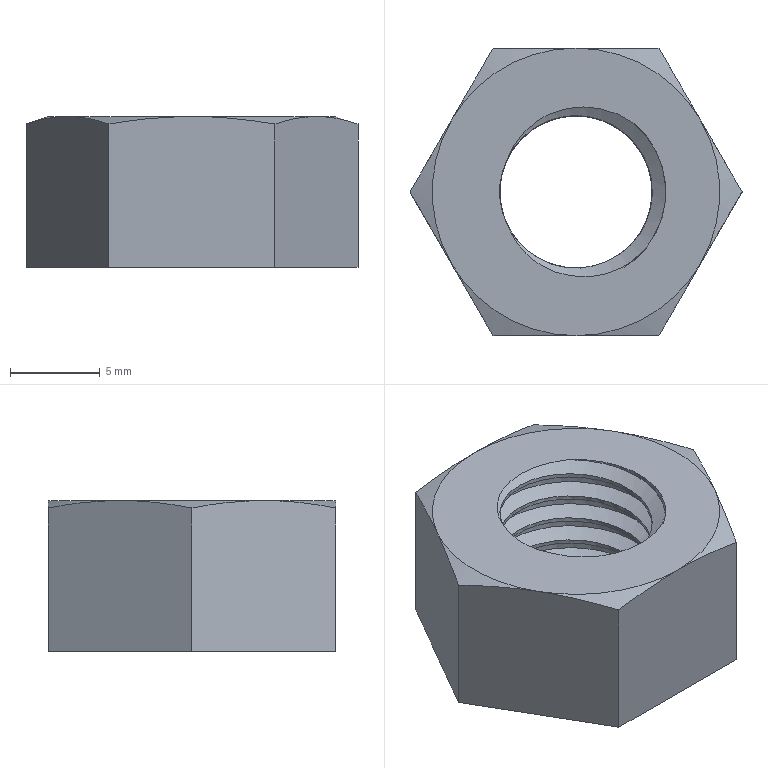Part | NX | features CHAMFER 1, CYLINDER 1, DATUM_CSYS 1, EXTRUDE 1, HOLE PACKAGE 1, SIMPLE HOLE 1, THREADS 1 | 1 solid | 19 faces | box 18.475 x 16 x 8.4 mm | volume 1288 mm3 | plane 9 | cone 6 | cylinder 2 | spline 2 | commonest cylinder face diameters 8.5 x1 10 x1
STEP:
#1=CARTESIAN_POINT('',(-4.619,-8.,0.));
#2=VERTEX_POINT('',#1);
#3=CARTESIAN_POINT('',(4.619,-8.,0.));
#4=VERTEX_POINT('',#3);
#5=CARTESIAN_POINT('',(-4.619,-8.,0.));
#6=DIRECTION('',(1.,0.,0.));
#7=VECTOR('',#6,1000.);
#8=LINE('',#5,#7);
#9=EDGE_CURVE('',#2,#4,#8,.T.);
#10=ORIENTED_EDGE('',*,*,#9,.F.);
#11=CARTESIAN_POINT('',(-9.238,0.,0.));
#12=VERTEX_POINT('',#11);
#13=CARTESIAN_POINT('',(-9.238,0.,0.));
#14=DIRECTION('',(0.5,-0.866,0.));
#15=VECTOR('',#14,1000.);
#16=LINE('',#13,#15);
#17=EDGE_CURVE('',#12,#2,#16,.T.);
#18=ORIENTED_EDGE('',*,*,#17,.F.);
#19=CARTESIAN_POINT('',(-4.619,8.,0.));
#20=VERTEX_POINT('',#19);
#21=CARTESIAN_POINT('',(-4.619,8.,0.));
#22=DIRECTION('',(-0.5,-0.866,0.));
#23=VECTOR('',#22,1000.);
#24=LINE('',#21,#23);
#25=EDGE_CURVE('',#20,#12,#24,.T.);
#26=ORIENTED_EDGE('',*,*,#25,.F.);
#27=CARTESIAN_POINT('',(4.619,8.,0.));
#28=VERTEX_POINT('',#27);
#29=CARTESIAN_POINT('',(4.619,8.,0.));
#30=DIRECTION('',(-1.,0.,0.));
#31=VECTOR('',#30,1000.);
#32=LINE('',#29,#31);
#33=EDGE_CURVE('',#28,#20,#32,.T.);
#34=ORIENTED_EDGE('',*,*,#33,.F.);
#35=CARTESIAN_POINT('',(9.238,0.,0.));
#36=VERTEX_POINT('',#35);
#37=CARTESIAN_POINT('',(9.238,0.,0.));
#38=DIRECTION('',(-0.5,0.866,0.));
#39=VECTOR('',#38,1000.);
#40=LINE('',#37,#39);
#41=EDGE_CURVE('',#36,#28,#40,.T.);
#42=ORIENTED_EDGE('',*,*,#41,.F.);
#43=CARTESIAN_POINT('',(4.619,-8.,0.));
#44=DIRECTION('',(0.5,0.866,0.));
#45=VECTOR('',#44,1000.);
#46=LINE('',#43,#45);
#47=EDGE_CURVE('',#4,#36,#46,.T.);
#48=ORIENTED_EDGE('',*,*,#47,.F.);
#49=EDGE_LOOP('',(#10,#18,#26,#34,#42,#48));
#50=FACE_BOUND('',#49,.T.);
#51=CARTESIAN_POINT('',(1.179,-4.083,0.));
#52=VERTEX_POINT('',#51);
#53=CARTESIAN_POINT('',(1.977,-3.762,0.));
#54=VERTEX_POINT('',#53);
#55=CARTESIAN_POINT('',(0.,0.,0.));
#56=DIRECTION('',(0.,0.,-1.));
#57=DIRECTION('',(-1.,0.,0.));
#58=AXIS2_PLACEMENT_3D('',#55,#56,#57);
#59=CIRCLE('',#58,4.25);
#60=EDGE_CURVE('',#52,#54,#59,.T.);
#61=ORIENTED_EDGE('',*,*,#60,.F.);
#62=CARTESIAN_POINT('',(1.202,-4.164,0.));
#63=VERTEX_POINT('',#62);
#64=CARTESIAN_POINT('',(0.,0.,0.));
#65=DIRECTION('',(0.2773,-0.9608,0.));
#66=VECTOR('',#65,1000.);
#67=LINE('',#64,#66);
#68=EDGE_CURVE('',#52,#63,#67,.T.);
#69=ORIENTED_EDGE('',*,*,#68,.T.);
#70=CARTESIAN_POINT('',(1.977,-3.762,0.));
#71=CARTESIAN_POINT('',(1.733,-3.923,0.));
#72=CARTESIAN_POINT('',(1.474,-4.056,0.));
#73=CARTESIAN_POINT('',(1.202,-4.164,0.));
#74=B_SPLINE_CURVE_WITH_KNOTS('',3,(#70,#71,#72,#73),.UNSPECIFIED.,.F.,.F.,(4,4),(0.0001042,0.0009768),.UNSPECIFIED.);
#75=EDGE_CURVE('',#54,#63,#74,.T.);
#76=ORIENTED_EDGE('',*,*,#75,.F.);
#77=EDGE_LOOP('',(#61,#69,#76));
#78=FACE_BOUND('',#77,.T.);
#79=CARTESIAN_POINT('',(0.,0.,0.));
#80=DIRECTION('',(0.,0.,-1.));
#81=DIRECTION('',(-1.,0.,0.));
#82=AXIS2_PLACEMENT_3D('',#79,#80,#81);
#83=PLANE('',#82);
#84=ADVANCED_FACE('',(#50,#78),#83,.T.);
#85=CARTESIAN_POINT('',(6.928,-4.,8.4));
#86=VERTEX_POINT('',#85);
#87=CARTESIAN_POINT('',(6.928,4.,8.4));
#88=VERTEX_POINT('',#87);
#89=CARTESIAN_POINT('',(0.,0.,8.4));
#90=DIRECTION('',(0.,0.,1.));
#91=DIRECTION('',(1.,0.,0.));
#92=AXIS2_PLACEMENT_3D('',#89,#90,#91);
#93=CIRCLE('',#92,8.);
#94=EDGE_CURVE('',#86,#88,#93,.T.);
#95=ORIENTED_EDGE('',*,*,#94,.F.);
#96=CARTESIAN_POINT('',(9.238,0.,7.987));
#97=VERTEX_POINT('',#96);
#98=CARTESIAN_POINT('',(6.928,-4.,8.4));
#99=CARTESIAN_POINT('',(7.698,-2.667,8.4));
#100=CARTESIAN_POINT('',(8.468,-1.333,8.244));
#101=CARTESIAN_POINT('',(9.238,0.,7.987));
#102=B_SPLINE_CURVE_WITH_KNOTS('',3,(#98,#99,#100,#101),.UNSPECIFIED.,.F.,.F.,(4,4),(0.004619,0.009238),.UNSPECIFIED.);
#103=EDGE_CURVE('',#86,#97,#102,.T.);
#104=ORIENTED_EDGE('',*,*,#103,.T.);
#105=CARTESIAN_POINT('',(9.238,0.,7.987));
#106=CARTESIAN_POINT('',(8.468,1.333,8.244));
#107=CARTESIAN_POINT('',(7.698,2.667,8.4));
#108=CARTESIAN_POINT('',(6.928,4.,8.4));
#109=B_SPLINE_CURVE_WITH_KNOTS('',3,(#105,#106,#107,#108),.UNSPECIFIED.,.F.,.F.,(4,4),(0.000000231,0.004619),.UNSPECIFIED.);
#110=EDGE_CURVE('',#97,#88,#109,.T.);
#111=ORIENTED_EDGE('',*,*,#110,.T.);
#112=EDGE_LOOP('',(#95,#104,#111));
#113=FACE_BOUND('',#112,.T.);
#114=CARTESIAN_POINT('',(0.,0.,7.4));
#115=DIRECTION('',(0.,0.,-1.));
#116=DIRECTION('',(-1.,0.,0.));
#117=AXIS2_PLACEMENT_3D('',#114,#115,#116);
#118=CONICAL_SURFACE('',#117,11.,1.249);
#119=ADVANCED_FACE('',(#113),#118,.T.);
#120=CARTESIAN_POINT('',(0.,-8.,8.4));
#121=VERTEX_POINT('',#120);
#122=CARTESIAN_POINT('',(0.,0.,8.4));
#123=DIRECTION('',(0.,0.,1.));
#124=DIRECTION('',(1.,0.,0.));
#125=AXIS2_PLACEMENT_3D('',#122,#123,#124);
#126=CIRCLE('',#125,8.);
#127=EDGE_CURVE('',#121,#86,#126,.T.);
#128=ORIENTED_EDGE('',*,*,#127,.F.);
#129=CARTESIAN_POINT('',(4.619,-8.,7.987));
#130=VERTEX_POINT('',#129);
#131=CARTESIAN_POINT('',(0.,-8.,8.4));
#132=CARTESIAN_POINT('',(1.544,-8.,8.4));
#133=CARTESIAN_POINT('',(3.083,-8.,8.243));
#134=CARTESIAN_POINT('',(4.619,-8.,7.987));
#135=B_SPLINE_CURVE_WITH_KNOTS('',3,(#131,#132,#133,#134),.UNSPECIFIED.,.F.,.F.,(4,4),(0.01252,0.01719),.UNSPECIFIED.);
#136=EDGE_CURVE('',#121,#130,#135,.T.);
#137=ORIENTED_EDGE('',*,*,#136,.T.);
#138=CARTESIAN_POINT('',(4.619,-8.,7.987));
#139=CARTESIAN_POINT('',(5.389,-6.667,8.244));
#140=CARTESIAN_POINT('',(6.158,-5.333,8.4));
#141=CARTESIAN_POINT('',(6.928,-4.,8.4));
#142=B_SPLINE_CURVE_WITH_KNOTS('',3,(#138,#139,#140,#141),.UNSPECIFIED.,.F.,.F.,(4,4),(0.000000231,0.004619),.UNSPECIFIED.);
#143=EDGE_CURVE('',#130,#86,#142,.T.);
#144=ORIENTED_EDGE('',*,*,#143,.T.);
#145=EDGE_LOOP('',(#128,#137,#144));
#146=FACE_BOUND('',#145,.T.);
#147=CARTESIAN_POINT('',(0.,0.,7.4));
#148=DIRECTION('',(0.,0.,-1.));
#149=DIRECTION('',(-1.,0.,0.));
#150=AXIS2_PLACEMENT_3D('',#147,#148,#149);
#151=CONICAL_SURFACE('',#150,11.,1.249);
#152=ADVANCED_FACE('',(#146),#151,.T.);
#153=CARTESIAN_POINT('',(-6.928,4.,8.4));
#154=VERTEX_POINT('',#153);
#155=CARTESIAN_POINT('',(-6.928,-4.,8.4));
#156=VERTEX_POINT('',#155);
#157=CARTESIAN_POINT('',(0.,0.,8.4));
#158=DIRECTION('',(0.,0.,1.));
#159=DIRECTION('',(1.,0.,0.));
#160=AXIS2_PLACEMENT_3D('',#157,#158,#159);
#161=CIRCLE('',#160,8.);
#162=EDGE_CURVE('',#154,#156,#161,.T.);
#163=ORIENTED_EDGE('',*,*,#162,.F.);
#164=CARTESIAN_POINT('',(-9.238,0.,7.987));
#165=VERTEX_POINT('',#164);
#166=CARTESIAN_POINT('',(-6.928,4.,8.4));
#167=CARTESIAN_POINT('',(-7.698,2.667,8.4));
#168=CARTESIAN_POINT('',(-8.468,1.333,8.244));
#169=CARTESIAN_POINT('',(-9.238,0.,7.987));
#170=B_SPLINE_CURVE_WITH_KNOTS('',3,(#166,#167,#168,#169),.UNSPECIFIED.,.F.,.F.,(4,4),(0.004619,0.009238),.UNSPECIFIED.);
#171=EDGE_CURVE('',#154,#165,#170,.T.);
#172=ORIENTED_EDGE('',*,*,#171,.T.);
#173=CARTESIAN_POINT('',(-9.238,0.,7.987));
#174=CARTESIAN_POINT('',(-8.468,-1.333,8.244));
#175=CARTESIAN_POINT('',(-7.698,-2.667,8.4));
#176=CARTESIAN_POINT('',(-6.928,-4.,8.4));
#177=B_SPLINE_CURVE_WITH_KNOTS('',3,(#173,#174,#175,#176),.UNSPECIFIED.,.F.,.F.,(4,4),(0.000000231,0.004619),.UNSPECIFIED.);
#178=EDGE_CURVE('',#165,#156,#177,.T.);
#179=ORIENTED_EDGE('',*,*,#178,.T.);
#180=EDGE_LOOP('',(#163,#172,#179));
#181=FACE_BOUND('',#180,.T.);
#182=CARTESIAN_POINT('',(0.,0.,7.4));
#183=DIRECTION('',(0.,0.,-1.));
#184=DIRECTION('',(-1.,0.,0.));
#185=AXIS2_PLACEMENT_3D('',#182,#183,#184);
#186=CONICAL_SURFACE('',#185,11.,1.249);
#187=ADVANCED_FACE('',(#181),#186,.T.);
#188=CARTESIAN_POINT('',(0.,8.,8.4));
#189=VERTEX_POINT('',#188);
#190=CARTESIAN_POINT('',(0.,0.,8.4));
#191=DIRECTION('',(0.,0.,1.));
#192=DIRECTION('',(1.,0.,0.));
#193=AXIS2_PLACEMENT_3D('',#190,#191,#192);
#194=CIRCLE('',#193,8.);
#195=EDGE_CURVE('',#189,#154,#194,.T.);
#196=ORIENTED_EDGE('',*,*,#195,.F.);
#197=CARTESIAN_POINT('',(-4.619,8.,7.987));
#198=VERTEX_POINT('',#197);
#199=CARTESIAN_POINT('',(-4.619,8.,7.987));
#200=CARTESIAN_POINT('',(-3.087,8.,8.243));
#201=CARTESIAN_POINT('',(-1.537,8.,8.4));
#202=CARTESIAN_POINT('',(0.,8.,8.4));
#203=B_SPLINE_CURVE_WITH_KNOTS('',3,(#199,#200,#201,#202),.UNSPECIFIED.,.F.,.F.,(4,4),(0.007866,0.01252),.UNSPECIFIED.);
#204=EDGE_CURVE('',#189,#198,#203,.F.);
#205=ORIENTED_EDGE('',*,*,#204,.T.);
#206=CARTESIAN_POINT('',(-4.619,8.,7.987));
#207=CARTESIAN_POINT('',(-5.389,6.667,8.244));
#208=CARTESIAN_POINT('',(-6.158,5.333,8.4));
#209=CARTESIAN_POINT('',(-6.928,4.,8.4));
#210=B_SPLINE_CURVE_WITH_KNOTS('',3,(#206,#207,#208,#209),.UNSPECIFIED.,.F.,.F.,(4,4),(0.000000231,0.004619),.UNSPECIFIED.);
#211=EDGE_CURVE('',#198,#154,#210,.T.);
#212=ORIENTED_EDGE('',*,*,#211,.T.);
#213=EDGE_LOOP('',(#196,#205,#212));
#214=FACE_BOUND('',#213,.T.);
#215=CARTESIAN_POINT('',(0.,0.,7.4));
#216=DIRECTION('',(0.,0.,-1.));
#217=DIRECTION('',(-1.,0.,0.));
#218=AXIS2_PLACEMENT_3D('',#215,#216,#217);
#219=CONICAL_SURFACE('',#218,11.,1.249);
#220=ADVANCED_FACE('',(#214),#219,.T.);
#221=CARTESIAN_POINT('',(0.,0.,8.4));
#222=DIRECTION('',(0.,0.,1.));
#223=DIRECTION('',(1.,0.,0.));
#224=AXIS2_PLACEMENT_3D('',#221,#222,#223);
#225=CIRCLE('',#224,8.);
#226=EDGE_CURVE('',#88,#189,#225,.T.);
#227=ORIENTED_EDGE('',*,*,#226,.F.);
#228=CARTESIAN_POINT('',(4.619,8.,7.987));
#229=VERTEX_POINT('',#228);
#230=CARTESIAN_POINT('',(6.928,4.,8.4));
#231=CARTESIAN_POINT('',(6.158,5.333,8.4));
#232=CARTESIAN_POINT('',(5.389,6.667,8.244));
#233=CARTESIAN_POINT('',(4.619,8.,7.987));
#234=B_SPLINE_CURVE_WITH_KNOTS('',3,(#230,#231,#232,#233),.UNSPECIFIED.,.F.,.F.,(4,4),(0.004619,0.009238),.UNSPECIFIED.);
#235=EDGE_CURVE('',#88,#229,#234,.T.);
#236=ORIENTED_EDGE('',*,*,#235,.T.);
#237=CARTESIAN_POINT('',(0.,8.,8.4));
#238=CARTESIAN_POINT('',(1.544,8.,8.4));
#239=CARTESIAN_POINT('',(3.083,8.,8.243));
#240=CARTESIAN_POINT('',(4.619,8.,7.987));
#241=B_SPLINE_CURVE_WITH_KNOTS('',3,(#237,#238,#239,#240),.UNSPECIFIED.,.F.,.F.,(4,4),(0.01252,0.01719),.UNSPECIFIED.);
#242=EDGE_CURVE('',#229,#189,#241,.F.);
#243=ORIENTED_EDGE('',*,*,#242,.T.);
#244=EDGE_LOOP('',(#227,#236,#243));
#245=FACE_BOUND('',#244,.T.);
#246=CARTESIAN_POINT('',(0.,0.,7.4));
#247=DIRECTION('',(0.,0.,-1.));
#248=DIRECTION('',(-1.,0.,0.));
#249=AXIS2_PLACEMENT_3D('',#246,#247,#248);
#250=CONICAL_SURFACE('',#249,11.,1.249);
#251=ADVANCED_FACE('',(#245),#250,.T.);
#252=CARTESIAN_POINT('',(3.228,3.819,8.4));
#253=VERTEX_POINT('',#252);
#254=CARTESIAN_POINT('',(-3.811,1.881,8.4));
#255=VERTEX_POINT('',#254);
#256=CARTESIAN_POINT('',(3.228,3.819,8.4));
#257=CARTESIAN_POINT('',(2.076,4.639,8.4));
#258=CARTESIAN_POINT('',(-0.936,5.227,8.4));
#259=CARTESIAN_POINT('',(-3.309,3.206,8.4));
#260=CARTESIAN_POINT('',(-3.811,1.881,8.4));
#261=B_SPLINE_CURVE_WITH_KNOTS('',3,(#256,#257,#258,#259,#260),.UNSPECIFIED.,.F.,.F.,(4,1,4),(0.00005872,0.004248,0.008437),.UNSPECIFIED.);
#262=EDGE_CURVE('',#253,#255,#261,.T.);
#263=ORIENTED_EDGE('',*,*,#262,.F.);
#264=CARTESIAN_POINT('',(3.228,-3.819,8.4));
#265=VERTEX_POINT('',#264);
#266=CARTESIAN_POINT('',(0.,0.,8.4));
#267=DIRECTION('',(0.,0.,1.));
#268=DIRECTION('',(1.,0.,0.));
#269=AXIS2_PLACEMENT_3D('',#266,#267,#268);
#270=CIRCLE('',#269,5.);
#271=EDGE_CURVE('',#265,#253,#270,.T.);
#272=ORIENTED_EDGE('',*,*,#271,.F.);
#273=CARTESIAN_POINT('',(-3.811,-1.881,8.4));
#274=VERTEX_POINT('',#273);
#275=CARTESIAN_POINT('',(-3.811,-1.881,8.4));
#276=CARTESIAN_POINT('',(-3.311,-3.202,8.4));
#277=CARTESIAN_POINT('',(-0.9386,-5.229,8.4));
#278=CARTESIAN_POINT('',(2.077,-4.638,8.4));
#279=CARTESIAN_POINT('',(3.228,-3.819,8.4));
#280=B_SPLINE_CURVE_WITH_KNOTS('',3,(#275,#276,#277,#278,#279),.UNSPECIFIED.,.F.,.F.,(4,1,4),(0.0001033,0.004312,0.00852),.UNSPECIFIED.);
#281=EDGE_CURVE('',#274,#265,#280,.T.);
#282=ORIENTED_EDGE('',*,*,#281,.F.);
#283=CARTESIAN_POINT('',(0.,0.,8.4));
#284=DIRECTION('',(0.,0.,-1.));
#285=DIRECTION('',(-1.,0.,0.));
#286=AXIS2_PLACEMENT_3D('',#283,#284,#285);
#287=CIRCLE('',#286,4.25);
#288=EDGE_CURVE('',#274,#255,#287,.T.);
#289=ORIENTED_EDGE('',*,*,#288,.T.);
#290=EDGE_LOOP('',(#263,#272,#282,#289));
#291=FACE_BOUND('',#290,.T.);
#292=ORIENTED_EDGE('',*,*,#226,.T.);
#293=ORIENTED_EDGE('',*,*,#195,.T.);
#294=ORIENTED_EDGE('',*,*,#162,.T.);
#295=CARTESIAN_POINT('',(0.,0.,8.4));
#296=DIRECTION('',(0.,0.,1.));
#297=DIRECTION('',(1.,0.,0.));
#298=AXIS2_PLACEMENT_3D('',#295,#296,#297);
#299=CIRCLE('',#298,8.);
#300=EDGE_CURVE('',#156,#121,#299,.T.);
#301=ORIENTED_EDGE('',*,*,#300,.T.);
#302=ORIENTED_EDGE('',*,*,#127,.T.);
#303=ORIENTED_EDGE('',*,*,#94,.T.);
#304=EDGE_LOOP('',(#292,#293,#294,#301,#302,#303));
#305=FACE_BOUND('',#304,.T.);
#306=CARTESIAN_POINT('',(0.,0.,8.4));
#307=DIRECTION('',(0.,0.,1.));
#308=DIRECTION('',(1.,0.,0.));
#309=AXIS2_PLACEMENT_3D('',#306,#307,#308);
#310=PLANE('',#309);
#311=ADVANCED_FACE('',(#291,#305),#310,.T.);
#312=CARTESIAN_POINT('',(-4.619,-8.,7.987));
#313=VERTEX_POINT('',#312);
#314=CARTESIAN_POINT('',(-6.928,-4.,8.4));
#315=CARTESIAN_POINT('',(-6.158,-5.333,8.4));
#316=CARTESIAN_POINT('',(-5.389,-6.667,8.244));
#317=CARTESIAN_POINT('',(-4.619,-8.,7.987));
#318=B_SPLINE_CURVE_WITH_KNOTS('',3,(#314,#315,#316,#317),.UNSPECIFIED.,.F.,.F.,(4,4),(0.004619,0.009238),.UNSPECIFIED.);
#319=EDGE_CURVE('',#156,#313,#318,.T.);
#320=ORIENTED_EDGE('',*,*,#319,.T.);
#321=CARTESIAN_POINT('',(-4.619,-8.,7.987));
#322=CARTESIAN_POINT('',(-3.087,-8.,8.243));
#323=CARTESIAN_POINT('',(-1.537,-8.,8.4));
#324=CARTESIAN_POINT('',(0.,-8.,8.4));
#325=B_SPLINE_CURVE_WITH_KNOTS('',3,(#321,#322,#323,#324),.UNSPECIFIED.,.F.,.F.,(4,4),(0.007866,0.01252),.UNSPECIFIED.);
#326=EDGE_CURVE('',#313,#121,#325,.T.);
#327=ORIENTED_EDGE('',*,*,#326,.T.);
#328=ORIENTED_EDGE('',*,*,#300,.F.);
#329=EDGE_LOOP('',(#320,#327,#328));
#330=FACE_BOUND('',#329,.T.);
#331=CARTESIAN_POINT('',(0.,0.,7.4));
#332=DIRECTION('',(0.,0.,-1.));
#333=DIRECTION('',(-1.,0.,0.));
#334=AXIS2_PLACEMENT_3D('',#331,#332,#333);
#335=CONICAL_SURFACE('',#334,11.,1.249);
#336=ADVANCED_FACE('',(#330),#335,.T.);
#337=ORIENTED_EDGE('',*,*,#326,.F.);
#338=CARTESIAN_POINT('',(-4.619,-8.,0.));
#339=DIRECTION('',(0.,0.,1.));
#340=VECTOR('',#339,1000.);
#341=LINE('',#338,#340);
#342=EDGE_CURVE('',#2,#313,#341,.T.);
#343=ORIENTED_EDGE('',*,*,#342,.F.);
#344=ORIENTED_EDGE('',*,*,#9,.T.);
#345=CARTESIAN_POINT('',(4.619,-8.,0.));
#346=DIRECTION('',(0.,0.,1.));
#347=VECTOR('',#346,1000.);
#348=LINE('',#345,#347);
#349=EDGE_CURVE('',#4,#130,#348,.T.);
#350=ORIENTED_EDGE('',*,*,#349,.T.);
#351=ORIENTED_EDGE('',*,*,#136,.F.);
#352=EDGE_LOOP('',(#337,#343,#344,#350,#351));
#353=FACE_BOUND('',#352,.T.);
#354=CARTESIAN_POINT('',(-4.619,-8.,0.));
#355=DIRECTION('',(0.,-1.,0.));
#356=DIRECTION('',(1.,0.,0.));
#357=AXIS2_PLACEMENT_3D('',#354,#355,#356);
#358=PLANE('',#357);
#359=ADVANCED_FACE('',(#353),#358,.T.);
#360=ORIENTED_EDGE('',*,*,#143,.F.);
#361=ORIENTED_EDGE('',*,*,#349,.F.);
#362=ORIENTED_EDGE('',*,*,#47,.T.);
#363=CARTESIAN_POINT('',(9.238,0.,0.));
#364=DIRECTION('',(0.,0.,1.));
#365=VECTOR('',#364,1000.);
#366=LINE('',#363,#365);
#367=EDGE_CURVE('',#36,#97,#366,.T.);
#368=ORIENTED_EDGE('',*,*,#367,.T.);
#369=ORIENTED_EDGE('',*,*,#103,.F.);
#370=EDGE_LOOP('',(#360,#361,#362,#368,#369));
#371=FACE_BOUND('',#370,.T.);
#372=CARTESIAN_POINT('',(4.619,-8.,0.));
#373=DIRECTION('',(0.866,-0.5,0.));
#374=DIRECTION('',(0.5,0.866,0.));
#375=AXIS2_PLACEMENT_3D('',#372,#373,#374);
#376=PLANE('',#375);
#377=ADVANCED_FACE('',(#371),#376,.T.);
#378=ORIENTED_EDGE('',*,*,#110,.F.);
#379=ORIENTED_EDGE('',*,*,#367,.F.);
#380=ORIENTED_EDGE('',*,*,#41,.T.);
#381=CARTESIAN_POINT('',(4.619,8.,0.));
#382=DIRECTION('',(0.,0.,1.));
#383=VECTOR('',#382,1000.);
#384=LINE('',#381,#383);
#385=EDGE_CURVE('',#28,#229,#384,.T.);
#386=ORIENTED_EDGE('',*,*,#385,.T.);
#387=ORIENTED_EDGE('',*,*,#235,.F.);
#388=EDGE_LOOP('',(#378,#379,#380,#386,#387));
#389=FACE_BOUND('',#388,.T.);
#390=CARTESIAN_POINT('',(9.238,0.,0.));
#391=DIRECTION('',(0.866,0.5,0.));
#392=DIRECTION('',(-0.5,0.866,0.));
#393=AXIS2_PLACEMENT_3D('',#390,#391,#392);
#394=PLANE('',#393);
#395=ADVANCED_FACE('',(#389),#394,.T.);
#396=ORIENTED_EDGE('',*,*,#242,.F.);
#397=ORIENTED_EDGE('',*,*,#385,.F.);
#398=ORIENTED_EDGE('',*,*,#33,.T.);
#399=CARTESIAN_POINT('',(-4.619,8.,0.));
#400=DIRECTION('',(0.,0.,1.));
#401=VECTOR('',#400,1000.);
#402=LINE('',#399,#401);
#403=EDGE_CURVE('',#20,#198,#402,.T.);
#404=ORIENTED_EDGE('',*,*,#403,.T.);
#405=ORIENTED_EDGE('',*,*,#204,.F.);
#406=EDGE_LOOP('',(#396,#397,#398,#404,#405));
#407=FACE_BOUND('',#406,.T.);
#408=CARTESIAN_POINT('',(4.619,8.,0.));
#409=DIRECTION('',(0.,1.,0.));
#410=DIRECTION('',(-1.,0.,0.));
#411=AXIS2_PLACEMENT_3D('',#408,#409,#410);
#412=PLANE('',#411);
#413=ADVANCED_FACE('',(#407),#412,.T.);
#414=ORIENTED_EDGE('',*,*,#211,.F.);
#415=ORIENTED_EDGE('',*,*,#403,.F.);
#416=ORIENTED_EDGE('',*,*,#25,.T.);
#417=CARTESIAN_POINT('',(-9.238,0.,0.));
#418=DIRECTION('',(0.,0.,1.));
#419=VECTOR('',#418,1000.);
#420=LINE('',#417,#419);
#421=EDGE_CURVE('',#12,#165,#420,.T.);
#422=ORIENTED_EDGE('',*,*,#421,.T.);
#423=ORIENTED_EDGE('',*,*,#171,.F.);
#424=EDGE_LOOP('',(#414,#415,#416,#422,#423));
#425=FACE_BOUND('',#424,.T.);
#426=CARTESIAN_POINT('',(-4.619,8.,0.));
#427=DIRECTION('',(-0.866,0.5,0.));
#428=DIRECTION('',(-0.5,-0.866,0.));
#429=AXIS2_PLACEMENT_3D('',#426,#427,#428);
#430=PLANE('',#429);
#431=ADVANCED_FACE('',(#425),#430,.T.);
#432=ORIENTED_EDGE('',*,*,#178,.F.);
#433=ORIENTED_EDGE('',*,*,#421,.F.);
#434=ORIENTED_EDGE('',*,*,#17,.T.);
#435=ORIENTED_EDGE('',*,*,#342,.T.);
#436=ORIENTED_EDGE('',*,*,#319,.F.);
#437=EDGE_LOOP('',(#432,#433,#434,#435,#436));
#438=FACE_BOUND('',#437,.T.);
#439=CARTESIAN_POINT('',(-9.238,0.,0.));
#440=DIRECTION('',(-0.866,-0.5,0.));
#441=DIRECTION('',(0.5,-0.866,0.));
#442=AXIS2_PLACEMENT_3D('',#439,#440,#441);
#443=PLANE('',#442);
#444=ADVANCED_FACE('',(#438),#443,.T.);
#445=ORIENTED_EDGE('',*,*,#60,.T.);
#446=CARTESIAN_POINT('',(1.977,-3.762,0.));
#447=CARTESIAN_POINT('',(3.369,-3.031,0.08878));
#448=CARTESIAN_POINT('',(5.184,0.06523,0.2621));
#449=CARTESIAN_POINT('',(2.302,4.66,0.5252));
#450=CARTESIAN_POINT('',(-3.109,4.164,0.7876));
#451=CARTESIAN_POINT('',(-5.12,-0.8825,1.05));
#452=CARTESIAN_POINT('',(-1.54,-4.961,1.313));
#453=CARTESIAN_POINT('',(3.72,-3.627,1.575));
#454=CARTESIAN_POINT('',(4.921,1.669,1.838));
#455=CARTESIAN_POINT('',(0.7438,5.142,2.1));
#456=CARTESIAN_POINT('',(-4.242,2.998,2.363));
#457=CARTESIAN_POINT('',(-4.599,-2.416,2.625));
#458=CARTESIAN_POINT('',(0.06565,-5.196,2.887));
#459=CARTESIAN_POINT('',(4.66,-2.297,3.15));
#460=CARTESIAN_POINT('',(4.163,3.107,3.413));
#461=CARTESIAN_POINT('',(-0.8754,5.121,3.675));
#462=CARTESIAN_POINT('',(-4.962,1.544,3.938));
#463=CARTESIAN_POINT('',(-3.626,-3.722,4.2));
#464=CARTESIAN_POINT('',(1.667,-4.92,4.462));
#465=CARTESIAN_POINT('',(5.141,-0.751,4.725));
#466=CARTESIAN_POINT('',(3.002,4.242,4.988));
#467=CARTESIAN_POINT('',(-2.418,4.599,5.25));
#468=CARTESIAN_POINT('',(-5.194,-0.06405,5.512));
#469=CARTESIAN_POINT('',(-2.304,-4.657,5.775));
#470=CARTESIAN_POINT('',(3.106,-4.166,6.038));
#471=CARTESIAN_POINT('',(5.121,0.8775,6.3));
#472=CARTESIAN_POINT('',(1.545,4.959,6.562));
#473=CARTESIAN_POINT('',(-3.716,3.631,6.825));
#474=CARTESIAN_POINT('',(-4.924,-1.666,7.087));
#475=CARTESIAN_POINT('',(-0.7415,-5.14,7.35));
#476=CARTESIAN_POINT('',(3.385,-3.361,7.569));
#477=CARTESIAN_POINT('',(4.458,-0.2923,7.744));
#478=CARTESIAN_POINT('',(3.959,2.073,7.875));
#479=CARTESIAN_POINT('',(2.29,3.838,8.006));
#480=CARTESIAN_POINT('',(-0.8428,4.688,8.181));
#481=CARTESIAN_POINT('',(-3.115,3.291,8.312));
#482=CARTESIAN_POINT('',(-3.811,1.881,8.4));
#483=B_SPLINE_CURVE_WITH_KNOTS('',3,(#446,#447,#448,#449,#450,#451,#452,#453,#454,#455,#456,#457,#458,#459,#460,#461,#462,#463,#464,#465,#466,#467,#468,#469,#470,#471,#472,#473,#474,#475,#476,#477,#478,#479,#480,#481,#482),.UNSPECIFIED.,.F.,.F.,(4,1,1,1,1,1,1,1,1,1,1,1,1,1,1,1,1,1,1,1,1,1,1,1,1,1,1,1,1,1,1,1,1,1,4),(0.,0.004678,0.009357,0.01404,0.01871,0.02339,0.02807,0.03275,0.03743,0.04211,0.04678,0.05146,0.05614,0.06082,0.0655,0.07018,0.07485,0.07953,0.08421,0.08889,0.09357,0.09825,0.1029,0.1076,0.1123,0.117,0.1216,0.1263,0.131,0.1357,0.138,0.1404,0.1427,0.145,0.1497),.UNSPECIFIED.);
#484=EDGE_CURVE('',#54,#255,#483,.T.);
#485=ORIENTED_EDGE('',*,*,#484,.T.);
#486=ORIENTED_EDGE('',*,*,#288,.F.);
#487=CARTESIAN_POINT('',(1.179,-4.083,1.233));
#488=VERTEX_POINT('',#487);
#489=CARTESIAN_POINT('',(-3.811,-1.881,8.4));
#490=CARTESIAN_POINT('',(-4.405,-0.6782,8.325));
#491=CARTESIAN_POINT('',(-4.36,2.267,8.176));
#492=CARTESIAN_POINT('',(-0.7489,4.865,7.952));
#493=CARTESIAN_POINT('',(3.482,3.477,7.728));
#494=CARTESIAN_POINT('',(4.862,-0.7537,7.504));
#495=CARTESIAN_POINT('',(2.267,-4.366,7.28));
#496=CARTESIAN_POINT('',(-2.178,-4.412,7.056));
#497=CARTESIAN_POINT('',(-4.847,-0.8513,6.832));
#498=CARTESIAN_POINT('',(-3.551,3.407,6.608));
#499=CARTESIAN_POINT('',(0.6494,4.877,6.384));
#500=CARTESIAN_POINT('',(4.315,2.363,6.16));
#501=CARTESIAN_POINT('',(4.458,-2.083,5.936));
#502=CARTESIAN_POINT('',(0.9539,-4.828,5.712));
#503=CARTESIAN_POINT('',(-3.331,-3.622,5.488));
#504=CARTESIAN_POINT('',(-4.889,0.5432,5.264));
#505=CARTESIAN_POINT('',(-2.456,4.263,5.04));
#506=CARTESIAN_POINT('',(1.988,4.502,4.816));
#507=CARTESIAN_POINT('',(4.806,1.056,4.592));
#508=CARTESIAN_POINT('',(3.692,-3.252,4.368));
#509=CARTESIAN_POINT('',(-0.4359,-4.9,4.144));
#510=CARTESIAN_POINT('',(-4.211,-2.547,3.92));
#511=CARTESIAN_POINT('',(-4.543,1.892,3.696));
#512=CARTESIAN_POINT('',(-1.158,4.782,3.472));
#513=CARTESIAN_POINT('',(3.17,3.762,3.248));
#514=CARTESIAN_POINT('',(4.909,-0.33,3.025));
#515=CARTESIAN_POINT('',(2.636,-4.156,2.8));
#516=CARTESIAN_POINT('',(-1.795,-4.582,2.577));
#517=CARTESIAN_POINT('',(-4.756,-1.26,2.352));
#518=CARTESIAN_POINT('',(-3.83,3.087,2.129));
#519=CARTESIAN_POINT('',(0.2245,4.915,1.905));
#520=CARTESIAN_POINT('',(4.101,2.724,1.68));
#521=CARTESIAN_POINT('',(4.61,-1.7,1.456));
#522=CARTESIAN_POINT('',(2.468,-3.711,1.308));
#523=CARTESIAN_POINT('',(1.179,-4.083,1.233));
#524=B_SPLINE_CURVE_WITH_KNOTS('',3,(#489,#490,#491,#492,#493,#494,#495,#496,#497,#498,#499,#500,#501,#502,#503,#504,#505,#506,#507,#508,#509,#510,#511,#512,#513,#514,#515,#516,#517,#518,#519,#520,#521,#522,#523),.UNSPECIFIED.,.F.,.F.,(4,1,1,1,1,1,1,1,1,1,1,1,1,1,1,1,1,1,1,1,1,1,1,1,1,1,1,1,1,1,1,1,4),(0.,0.003992,0.007984,0.01198,0.01597,0.01996,0.02395,0.02794,0.03194,0.03593,0.03992,0.04391,0.0479,0.0519,0.05589,0.05988,0.06387,0.06786,0.07185,0.07585,0.07984,0.08383,0.08782,0.09181,0.09581,0.0998,0.1038,0.1078,0.1118,0.1158,0.1198,0.1238,0.1277),.UNSPECIFIED.);
#525=EDGE_CURVE('',#274,#488,#524,.T.);
#526=ORIENTED_EDGE('',*,*,#525,.T.);
#527=CARTESIAN_POINT('',(1.179,-4.083,8.4));
#528=DIRECTION('',(0.,0.,-1.));
#529=VECTOR('',#528,1000.);
#530=LINE('',#527,#529);
#531=EDGE_CURVE('',#52,#488,#530,.F.);
#532=ORIENTED_EDGE('',*,*,#531,.F.);
#533=EDGE_LOOP('',(#445,#485,#486,#526,#532));
#534=FACE_BOUND('',#533,.T.);
#535=CARTESIAN_POINT('',(0.,0.,8.4));
#536=DIRECTION('',(0.,0.,-1.));
#537=DIRECTION('',(-1.,0.,0.));
#538=AXIS2_PLACEMENT_3D('',#535,#536,#537);
#539=CYLINDRICAL_SURFACE('',#538,4.25);
#540=ADVANCED_FACE('',(#534),#539,.F.);
#541=ORIENTED_EDGE('',*,*,#281,.T.);
#542=CARTESIAN_POINT('',(1.387,-4.804,0.7995));
#543=VERTEX_POINT('',#542);
#544=CARTESIAN_POINT('',(1.387,-4.804,0.7995));
#545=CARTESIAN_POINT('',(2.995,-4.34,0.8799));
#546=CARTESIAN_POINT('',(5.628,-1.718,1.036));
#547=CARTESIAN_POINT('',(4.513,3.797,1.275));
#548=CARTESIAN_POINT('',(-0.7286,5.849,1.512));
#549=CARTESIAN_POINT('',(-5.302,2.576,1.75));
#550=CARTESIAN_POINT('',(-5.048,-3.045,1.987));
#551=CARTESIAN_POINT('',(-0.1952,-5.892,2.225));
#552=CARTESIAN_POINT('',(4.835,-3.372,2.462));
#553=CARTESIAN_POINT('',(5.461,2.219,2.7));
#554=CARTESIAN_POINT('',(1.112,5.789,2.937));
#555=CARTESIAN_POINT('',(-4.25,4.085,3.175));
#556=CARTESIAN_POINT('',(-5.741,-1.34,3.412));
#557=CARTESIAN_POINT('',(-2.002,-5.545,3.65));
#558=CARTESIAN_POINT('',(3.56,-4.698,3.887));
#559=CARTESIAN_POINT('',(5.879,0.4273,4.125));
#560=CARTESIAN_POINT('',(2.843,5.164,4.362));
#561=CARTESIAN_POINT('',(-2.782,5.197,4.6));
#562=CARTESIAN_POINT('',(-5.874,0.4975,4.837));
#563=CARTESIAN_POINT('',(-3.617,-4.655,5.075));
#564=CARTESIAN_POINT('',(1.933,-5.568,5.312));
#565=CARTESIAN_POINT('',(5.723,-1.412,5.55));
#566=CARTESIAN_POINT('',(4.301,4.031,5.787));
#567=CARTESIAN_POINT('',(-1.038,5.803,6.024));
#568=CARTESIAN_POINT('',(-5.432,2.289,6.263));
#569=CARTESIAN_POINT('',(-4.878,-3.309,6.499));
#570=CARTESIAN_POINT('',(0.119,-5.894,6.738));
#571=CARTESIAN_POINT('',(5.008,-3.11,6.975));
#572=CARTESIAN_POINT('',(5.335,2.507,7.213));
#573=CARTESIAN_POINT('',(0.8021,5.84,7.45));
#574=CARTESIAN_POINT('',(-4.461,3.853,7.688));
#575=CARTESIAN_POINT('',(-5.662,-1.645,7.925));
#576=CARTESIAN_POINT('',(-1.701,-5.641,8.163));
#577=CARTESIAN_POINT('',(1.963,-4.887,8.32));
#578=CARTESIAN_POINT('',(3.228,-3.819,8.4));
#579=B_SPLINE_CURVE_WITH_KNOTS('',3,(#544,#545,#546,#547,#548,#549,#550,#551,#552,#553,#554,#555,#556,#557,#558,#559,#560,#561,#562,#563,#564,#565,#566,#567,#568,#569,#570,#571,#572,#573,#574,#575,#576,#577,#578),.UNSPECIFIED.,.F.,.F.,(4,1,1,1,1,1,1,1,1,1,1,1,1,1,1,1,1,1,1,1,1,1,1,1,1,1,1,1,1,1,1,1,4),(0.,0.004957,0.009913,0.01487,0.01983,0.02478,0.02974,0.0347,0.03965,0.04461,0.04957,0.05452,0.05948,0.06443,0.06939,0.07435,0.0793,0.08426,0.08922,0.09417,0.09913,0.1041,0.109,0.114,0.119,0.1239,0.1289,0.1338,0.1388,0.1437,0.1487,0.1537,0.1586),.UNSPECIFIED.);
#580=EDGE_CURVE('',#265,#543,#579,.F.);
#581=ORIENTED_EDGE('',*,*,#580,.T.);
#582=CARTESIAN_POINT('',(1.455,-5.041,0.657));
#583=CARTESIAN_POINT('',(1.176,-4.074,1.238));
#584=B_SPLINE_CURVE_WITH_KNOTS('',1,(#582,#583),.UNSPECIFIED.,.F.,.F.,(2,2),(0.,1.),.PIECEWISE_BEZIER_KNOTS.);
#585=EDGE_CURVE('',#543,#488,#584,.T.);
#586=ORIENTED_EDGE('',*,*,#585,.T.);
#587=ORIENTED_EDGE('',*,*,#525,.F.);
#588=EDGE_LOOP('',(#541,#581,#586,#587));
#589=FACE_BOUND('',#588,.T.);
#590=CARTESIAN_POINT('',(3.898,-3.139,8.443));
#591=CARTESIAN_POINT('',(3.785,-3.279,8.434));
#592=CARTESIAN_POINT('',(3.228,-3.901,8.394));
#593=CARTESIAN_POINT('',(1.965,-4.744,8.323));
#594=CARTESIAN_POINT('',(0.,-5.135,8.23));
#595=CARTESIAN_POINT('',(-1.965,-4.744,8.136));
#596=CARTESIAN_POINT('',(-3.631,-3.631,8.042));
#597=CARTESIAN_POINT('',(-4.744,-1.965,7.948));
#598=CARTESIAN_POINT('',(-5.135,0.,7.855));
#599=CARTESIAN_POINT('',(-4.744,1.965,7.761));
#600=CARTESIAN_POINT('',(-3.631,3.631,7.667));
#601=CARTESIAN_POINT('',(-1.965,4.744,7.573));
#602=CARTESIAN_POINT('',(0.,5.135,7.48));
#603=CARTESIAN_POINT('',(1.965,4.744,7.386));
#604=CARTESIAN_POINT('',(3.631,3.631,7.292));
#605=CARTESIAN_POINT('',(4.744,1.965,7.198));
#606=CARTESIAN_POINT('',(5.135,0.,7.105));
#607=CARTESIAN_POINT('',(4.744,-1.965,7.011));
#608=CARTESIAN_POINT('',(3.631,-3.631,6.917));
#609=CARTESIAN_POINT('',(1.965,-4.744,6.823));
#610=CARTESIAN_POINT('',(0.,-5.135,6.73));
#611=CARTESIAN_POINT('',(-1.965,-4.744,6.636));
#612=CARTESIAN_POINT('',(-3.631,-3.631,6.542));
#613=CARTESIAN_POINT('',(-4.744,-1.965,6.448));
#614=CARTESIAN_POINT('',(-5.135,0.,6.355));
#615=CARTESIAN_POINT('',(-4.744,1.965,6.261));
#616=CARTESIAN_POINT('',(-3.631,3.631,6.167));
#617=CARTESIAN_POINT('',(-1.965,4.744,6.073));
#618=CARTESIAN_POINT('',(0.,5.135,5.98));
#619=CARTESIAN_POINT('',(1.965,4.744,5.886));
#620=CARTESIAN_POINT('',(3.631,3.631,5.792));
#621=CARTESIAN_POINT('',(4.744,1.965,5.698));
#622=CARTESIAN_POINT('',(5.135,0.,5.605));
#623=CARTESIAN_POINT('',(4.744,-1.965,5.511));
#624=CARTESIAN_POINT('',(3.631,-3.631,5.417));
#625=CARTESIAN_POINT('',(1.965,-4.744,5.323));
#626=CARTESIAN_POINT('',(0.,-5.135,5.23));
#627=CARTESIAN_POINT('',(-1.965,-4.744,5.136));
#628=CARTESIAN_POINT('',(-3.631,-3.631,5.042));
#629=CARTESIAN_POINT('',(-4.744,-1.965,4.948));
#630=CARTESIAN_POINT('',(-5.135,0.,4.855));
#631=CARTESIAN_POINT('',(-4.744,1.965,4.761));
#632=CARTESIAN_POINT('',(-3.631,3.631,4.667));
#633=CARTESIAN_POINT('',(-1.965,4.744,4.573));
#634=CARTESIAN_POINT('',(0.,5.135,4.48));
#635=CARTESIAN_POINT('',(1.965,4.744,4.386));
#636=CARTESIAN_POINT('',(3.631,3.631,4.292));
#637=CARTESIAN_POINT('',(4.744,1.965,4.198));
#638=CARTESIAN_POINT('',(5.135,0.,4.105));
#639=CARTESIAN_POINT('',(4.744,-1.965,4.011));
#640=CARTESIAN_POINT('',(3.631,-3.631,3.917));
#641=CARTESIAN_POINT('',(1.965,-4.744,3.823));
#642=CARTESIAN_POINT('',(0.,-5.135,3.73));
#643=CARTESIAN_POINT('',(-1.965,-4.744,3.636));
#644=CARTESIAN_POINT('',(-3.631,-3.631,3.542));
#645=CARTESIAN_POINT('',(-4.744,-1.965,3.448));
#646=CARTESIAN_POINT('',(-5.135,0.,3.355));
#647=CARTESIAN_POINT('',(-4.744,1.965,3.261));
#648=CARTESIAN_POINT('',(-3.631,3.631,3.167));
#649=CARTESIAN_POINT('',(-1.965,4.744,3.073));
#650=CARTESIAN_POINT('',(0.,5.135,2.98));
#651=CARTESIAN_POINT('',(1.965,4.744,2.886));
#652=CARTESIAN_POINT('',(3.631,3.631,2.792));
#653=CARTESIAN_POINT('',(4.744,1.965,2.698));
#654=CARTESIAN_POINT('',(5.135,0.,2.605));
#655=CARTESIAN_POINT('',(4.744,-1.965,2.511));
#656=CARTESIAN_POINT('',(3.631,-3.631,2.417));
#657=CARTESIAN_POINT('',(1.965,-4.744,2.323));
#658=CARTESIAN_POINT('',(0.,-5.135,2.23));
#659=CARTESIAN_POINT('',(-1.965,-4.744,2.136));
#660=CARTESIAN_POINT('',(-3.631,-3.631,2.042));
#661=CARTESIAN_POINT('',(-4.744,-1.965,1.948));
#662=CARTESIAN_POINT('',(-5.135,0.,1.855));
#663=CARTESIAN_POINT('',(-4.744,1.965,1.761));
#664=CARTESIAN_POINT('',(-3.631,3.631,1.667));
#665=CARTESIAN_POINT('',(-1.965,4.744,1.573));
#666=CARTESIAN_POINT('',(0.,5.135,1.48));
#667=CARTESIAN_POINT('',(1.965,4.744,1.386));
#668=CARTESIAN_POINT('',(3.631,3.631,1.292));
#669=CARTESIAN_POINT('',(4.744,1.965,1.198));
#670=CARTESIAN_POINT('',(5.135,0.,1.105));
#671=CARTESIAN_POINT('',(4.744,-1.965,1.011));
#672=CARTESIAN_POINT('',(3.631,-3.631,0.9172));
#673=CARTESIAN_POINT('',(2.363,-4.479,0.8458));
#674=CARTESIAN_POINT('',(1.567,-4.757,0.8057));
#675=CARTESIAN_POINT('',(1.388,-4.808,0.7968));
#676=CARTESIAN_POINT('',(3.306,-2.663,8.881));
#677=CARTESIAN_POINT('',(3.211,-2.781,8.873));
#678=CARTESIAN_POINT('',(2.738,-3.309,8.833));
#679=CARTESIAN_POINT('',(1.667,-4.024,8.762));
#680=CARTESIAN_POINT('',(0.,-4.356,8.668));
#681=CARTESIAN_POINT('',(-1.667,-4.024,8.575));
#682=CARTESIAN_POINT('',(-3.08,-3.08,8.481));
#683=CARTESIAN_POINT('',(-4.024,-1.667,8.387));
#684=CARTESIAN_POINT('',(-4.356,0.,8.293));
#685=CARTESIAN_POINT('',(-4.024,1.667,8.2));
#686=CARTESIAN_POINT('',(-3.08,3.08,8.106));
#687=CARTESIAN_POINT('',(-1.667,4.024,8.012));
#688=CARTESIAN_POINT('',(0.,4.356,7.918));
#689=CARTESIAN_POINT('',(1.667,4.024,7.825));
#690=CARTESIAN_POINT('',(3.08,3.08,7.731));
#691=CARTESIAN_POINT('',(4.024,1.667,7.637));
#692=CARTESIAN_POINT('',(4.356,0.,7.543));
#693=CARTESIAN_POINT('',(4.024,-1.667,7.45));
#694=CARTESIAN_POINT('',(3.08,-3.08,7.356));
#695=CARTESIAN_POINT('',(1.667,-4.024,7.262));
#696=CARTESIAN_POINT('',(0.,-4.356,7.168));
#697=CARTESIAN_POINT('',(-1.667,-4.024,7.075));
#698=CARTESIAN_POINT('',(-3.08,-3.08,6.981));
#699=CARTESIAN_POINT('',(-4.024,-1.667,6.887));
#700=CARTESIAN_POINT('',(-4.356,0.,6.793));
#701=CARTESIAN_POINT('',(-4.024,1.667,6.7));
#702=CARTESIAN_POINT('',(-3.08,3.08,6.606));
#703=CARTESIAN_POINT('',(-1.667,4.024,6.512));
#704=CARTESIAN_POINT('',(0.,4.356,6.418));
#705=CARTESIAN_POINT('',(1.667,4.024,6.325));
#706=CARTESIAN_POINT('',(3.08,3.08,6.231));
#707=CARTESIAN_POINT('',(4.024,1.667,6.137));
#708=CARTESIAN_POINT('',(4.356,0.,6.043));
#709=CARTESIAN_POINT('',(4.024,-1.667,5.95));
#710=CARTESIAN_POINT('',(3.08,-3.08,5.856));
#711=CARTESIAN_POINT('',(1.667,-4.024,5.762));
#712=CARTESIAN_POINT('',(0.,-4.356,5.668));
#713=CARTESIAN_POINT('',(-1.667,-4.024,5.575));
#714=CARTESIAN_POINT('',(-3.08,-3.08,5.481));
#715=CARTESIAN_POINT('',(-4.024,-1.667,5.387));
#716=CARTESIAN_POINT('',(-4.356,0.,5.293));
#717=CARTESIAN_POINT('',(-4.024,1.667,5.2));
#718=CARTESIAN_POINT('',(-3.08,3.08,5.106));
#719=CARTESIAN_POINT('',(-1.667,4.024,5.012));
#720=CARTESIAN_POINT('',(0.,4.356,4.918));
#721=CARTESIAN_POINT('',(1.667,4.024,4.825));
#722=CARTESIAN_POINT('',(3.08,3.08,4.731));
#723=CARTESIAN_POINT('',(4.024,1.667,4.637));
#724=CARTESIAN_POINT('',(4.356,0.,4.543));
#725=CARTESIAN_POINT('',(4.024,-1.667,4.45));
#726=CARTESIAN_POINT('',(3.08,-3.08,4.356));
#727=CARTESIAN_POINT('',(1.667,-4.024,4.262));
#728=CARTESIAN_POINT('',(0.,-4.356,4.168));
#729=CARTESIAN_POINT('',(-1.667,-4.024,4.075));
#730=CARTESIAN_POINT('',(-3.08,-3.08,3.981));
#731=CARTESIAN_POINT('',(-4.024,-1.667,3.887));
#732=CARTESIAN_POINT('',(-4.356,0.,3.793));
#733=CARTESIAN_POINT('',(-4.024,1.667,3.7));
#734=CARTESIAN_POINT('',(-3.08,3.08,3.606));
#735=CARTESIAN_POINT('',(-1.667,4.024,3.512));
#736=CARTESIAN_POINT('',(0.,4.356,3.418));
#737=CARTESIAN_POINT('',(1.667,4.024,3.325));
#738=CARTESIAN_POINT('',(3.08,3.08,3.231));
#739=CARTESIAN_POINT('',(4.024,1.667,3.137));
#740=CARTESIAN_POINT('',(4.356,0.,3.043));
#741=CARTESIAN_POINT('',(4.024,-1.667,2.95));
#742=CARTESIAN_POINT('',(3.08,-3.08,2.856));
#743=CARTESIAN_POINT('',(1.667,-4.024,2.762));
#744=CARTESIAN_POINT('',(0.,-4.356,2.668));
#745=CARTESIAN_POINT('',(-1.667,-4.024,2.575));
#746=CARTESIAN_POINT('',(-3.08,-3.08,2.481));
#747=CARTESIAN_POINT('',(-4.024,-1.667,2.387));
#748=CARTESIAN_POINT('',(-4.356,0.,2.293));
#749=CARTESIAN_POINT('',(-4.024,1.667,2.2));
#750=CARTESIAN_POINT('',(-3.08,3.08,2.106));
#751=CARTESIAN_POINT('',(-1.667,4.024,2.012));
#752=CARTESIAN_POINT('',(0.,4.356,1.918));
#753=CARTESIAN_POINT('',(1.667,4.024,1.825));
#754=CARTESIAN_POINT('',(3.08,3.08,1.731));
#755=CARTESIAN_POINT('',(4.024,1.667,1.637));
#756=CARTESIAN_POINT('',(4.356,0.,1.543));
#757=CARTESIAN_POINT('',(4.024,-1.667,1.45));
#758=CARTESIAN_POINT('',(3.08,-3.08,1.356));
#759=CARTESIAN_POINT('',(2.004,-3.799,1.284));
#760=CARTESIAN_POINT('',(1.329,-4.035,1.244));
#761=CARTESIAN_POINT('',(1.177,-4.079,1.235));
#762=B_SPLINE_SURFACE_WITH_KNOTS('',1,3,((#590,#591,#592,#593,#594,#595,#596,#597,#598,#599,#600,#601,#602,#603,#604,#605,#606,#607,#608,#609,#610,#611,#612,#613,#614,#615,#616,#617,#618,#619,#620,#621,#622,#623,#624,#625,#626,#627,#628,#629,#630,#631,#632,#633,#634,#635,#636,#637,#638,#639,#640,#641,#642,#643,#644,#645,#646,#647,#648,#649,#650,#651,#652,#653,#654,#655,#656,#657,#658,#659,#660,#661,#662,#663,#664,#665,#666,#667,#668,#669,#670,#671,#672,#673,#674,#675),(#676,#677,#678,#679,#680,#681,#682,#683,#684,#685,#686,#687,#688,#689,#690,#691,#692,#693,#694,#695,#696,#697,#698,#699,#700,#701,#702,#703,#704,#705,#706,#707,#708,#709,#710,#711,#712,#713,#714,#715,#716,#717,#718,#719,#720,#721,#722,#723,#724,#725,#726,#727,#728,#729,#730,#731,#732,#733,#734,#735,#736,#737,#738,#739,#740,#741,#742,#743,#744,#745,#746,#747,#748,#749,#750,#751,#752,#753,#754,#755,#756,#757,#758,#759,#760,#761)),.RULED_SURF.,.F.,.F.,.F.,(2,2),(4,1,1,1,1,1,1,1,1,1,1,1,1,1,1,1,1,1,1,1,1,1,1,1,1,1,1,1,1,1,1,1,1,1,1,1,1,1,1,1,1,1,1,1,1,1,1,1,1,1,1,1,1,1,1,1,1,1,1,1,1,1,1,1,1,1,1,1,1,1,1,1,1,1,1,1,1,1,1,1,1,1,1,4),(0.2404,0.9947),(0.1066,0.1095,0.1205,0.1315,0.1424,0.1534,0.1643,0.1753,0.1862,0.1972,0.2081,0.2191,0.2301,0.241,0.252,0.2629,0.2739,0.2848,0.2958,0.3067,0.3177,0.3286,0.3396,0.3506,0.3615,0.3725,0.3834,0.3944,0.4053,0.4163,0.4272,0.4382,0.4491,0.4601,0.4711,0.482,0.493,0.5039,0.5149,0.5258,0.5368,0.5477,0.5587,0.5696,0.5806,0.5916,0.6025,0.6135,0.6244,0.6354,0.6463,0.6573,0.6682,0.6792,0.6902,0.7011,0.7121,0.723,0.734,0.7449,0.7559,0.7668,0.7778,0.7887,0.7997,0.8107,0.8216,0.8326,0.8435,0.8545,0.8654,0.8764,0.8873,0.8983,0.9092,0.9202,0.9312,0.9421,0.9531,0.964,0.975,0.9859,0.9969,1.),.UNSPECIFIED.);
#763=ADVANCED_FACE('',(#589),#762,.F.);
#764=ORIENTED_EDGE('',*,*,#531,.T.);
#765=ORIENTED_EDGE('',*,*,#585,.F.);
#766=CARTESIAN_POINT('',(1.387,-4.804,0.3847));
#767=VERTEX_POINT('',#766);
#768=CARTESIAN_POINT('',(1.387,-4.804,9.15));
#769=DIRECTION('',(0.,0.,-1.));
#770=VECTOR('',#769,1000.);
#771=LINE('',#768,#770);
#772=EDGE_CURVE('',#767,#543,#771,.F.);
#773=ORIENTED_EDGE('',*,*,#772,.F.);
#774=CARTESIAN_POINT('',(1.176,-4.074,-0.05427));
#775=CARTESIAN_POINT('',(1.455,-5.041,0.5272));
#776=B_SPLINE_CURVE_WITH_KNOTS('',1,(#774,#775),.UNSPECIFIED.,.F.,.F.,(2,2),(0.,1.),.PIECEWISE_BEZIER_KNOTS.);
#777=EDGE_CURVE('',#63,#767,#776,.T.);
#778=ORIENTED_EDGE('',*,*,#777,.F.);
#779=ORIENTED_EDGE('',*,*,#68,.F.);
#780=EDGE_LOOP('',(#764,#765,#773,#778,#779));
#781=FACE_BOUND('',#780,.T.);
#782=CARTESIAN_POINT('',(1.176,-4.074,0.5921));
#783=DIRECTION('',(0.9608,0.2773,0.));
#784=DIRECTION('',(-0.2773,0.9608,0.));
#785=AXIS2_PLACEMENT_3D('',#782,#783,#784);
#786=PLANE('',#785);
#787=ADVANCED_FACE('',(#781),#786,.T.);
#788=ORIENTED_EDGE('',*,*,#262,.T.);
#789=ORIENTED_EDGE('',*,*,#484,.F.);
#790=ORIENTED_EDGE('',*,*,#75,.T.);
#791=ORIENTED_EDGE('',*,*,#777,.T.);
#792=CARTESIAN_POINT('',(3.228,3.819,8.4));
#793=CARTESIAN_POINT('',(4.561,2.692,8.316));
#794=CARTESIAN_POINT('',(5.903,-1.072,8.15));
#795=CARTESIAN_POINT('',(2.011,-5.659,7.899));
#796=CARTESIAN_POINT('',(-3.906,-4.561,7.648));
#797=CARTESIAN_POINT('',(-5.9,1.114,7.398));
#798=CARTESIAN_POINT('',(-1.973,5.67,7.147));
#799=CARTESIAN_POINT('',(3.932,4.537,6.897));
#800=CARTESIAN_POINT('',(5.893,-1.148,6.647));
#801=CARTESIAN_POINT('',(1.942,-5.681,6.396));
#802=CARTESIAN_POINT('',(-3.957,-4.515,6.146));
#803=CARTESIAN_POINT('',(-5.887,1.181,5.895));
#804=CARTESIAN_POINT('',(-1.909,5.693,5.645));
#805=CARTESIAN_POINT('',(3.986,4.491,5.394));
#806=CARTESIAN_POINT('',(5.879,-1.22,5.144));
#807=CARTESIAN_POINT('',(1.871,-5.705,4.893));
#808=CARTESIAN_POINT('',(-4.013,-4.465,4.643));
#809=CARTESIAN_POINT('',(-5.871,1.254,4.392));
#810=CARTESIAN_POINT('',(-1.839,5.715,4.142));
#811=CARTESIAN_POINT('',(4.038,4.443,3.891));
#812=CARTESIAN_POINT('',(5.865,-1.286,3.641));
#813=CARTESIAN_POINT('',(1.807,-5.726,3.39));
#814=CARTESIAN_POINT('',(-4.065,-4.419,3.14));
#815=CARTESIAN_POINT('',(-5.857,1.325,2.89));
#816=CARTESIAN_POINT('',(-1.769,5.738,2.639));
#817=CARTESIAN_POINT('',(4.093,4.393,2.388));
#818=CARTESIAN_POINT('',(5.848,-1.359,2.138));
#819=CARTESIAN_POINT('',(1.736,-5.747,1.888));
#820=CARTESIAN_POINT('',(-4.117,-4.37,1.637));
#821=CARTESIAN_POINT('',(-5.84,1.392,1.387));
#822=CARTESIAN_POINT('',(-1.705,5.757,1.136));
#823=CARTESIAN_POINT('',(4.147,4.347,0.8856));
#824=CARTESIAN_POINT('',(5.819,-1.433,0.6352));
#825=CARTESIAN_POINT('',(3.083,-4.314,0.4685));
#826=CARTESIAN_POINT('',(1.387,-4.804,0.3847));
#827=B_SPLINE_CURVE_WITH_KNOTS('',3,(#792,#793,#794,#795,#796,#797,#798,#799,#800,#801,#802,#803,#804,#805,#806,#807,#808,#809,#810,#811,#812,#813,#814,#815,#816,#817,#818,#819,#820,#821,#822,#823,#824,#825,#826),.UNSPECIFIED.,.F.,.F.,(4,1,1,1,1,1,1,1,1,1,1,1,1,1,1,1,1,1,1,1,1,1,1,1,1,1,1,1,1,1,1,1,4),(0.01132,0.01655,0.02178,0.027,0.03223,0.03746,0.04269,0.04791,0.05314,0.05837,0.06359,0.06882,0.07405,0.07927,0.0845,0.08973,0.09496,0.1002,0.1054,0.1106,0.1159,0.1211,0.1263,0.1315,0.1368,0.142,0.1472,0.1525,0.1577,0.1629,0.1681,0.1734,0.1786),.UNSPECIFIED.);
#828=EDGE_CURVE('',#767,#253,#827,.F.);
#829=ORIENTED_EDGE('',*,*,#828,.T.);
#830=EDGE_LOOP('',(#788,#789,#790,#791,#829));
#831=FACE_BOUND('',#830,.T.);
#832=CARTESIAN_POINT('',(-4.117,1.035,8.448));
#833=CARTESIAN_POINT('',(-4.067,1.236,8.436));
#834=CARTESIAN_POINT('',(-3.827,1.962,8.393));
#835=CARTESIAN_POINT('',(-3.08,3.08,8.319));
#836=CARTESIAN_POINT('',(-1.667,4.024,8.225));
#837=CARTESIAN_POINT('',(0.,4.356,8.132));
#838=CARTESIAN_POINT('',(1.667,4.024,8.038));
#839=CARTESIAN_POINT('',(3.08,3.08,7.944));
#840=CARTESIAN_POINT('',(4.024,1.667,7.85));
#841=CARTESIAN_POINT('',(4.356,0.,7.757));
#842=CARTESIAN_POINT('',(4.024,-1.667,7.663));
#843=CARTESIAN_POINT('',(3.08,-3.08,7.569));
#844=CARTESIAN_POINT('',(1.667,-4.024,7.475));
#845=CARTESIAN_POINT('',(0.,-4.356,7.382));
#846=CARTESIAN_POINT('',(-1.667,-4.024,7.288));
#847=CARTESIAN_POINT('',(-3.08,-3.08,7.194));
#848=CARTESIAN_POINT('',(-4.024,-1.667,7.1));
#849=CARTESIAN_POINT('',(-4.356,0.,7.007));
#850=CARTESIAN_POINT('',(-4.024,1.667,6.913));
#851=CARTESIAN_POINT('',(-3.08,3.08,6.819));
#852=CARTESIAN_POINT('',(-1.667,4.024,6.725));
#853=CARTESIAN_POINT('',(0.,4.356,6.632));
#854=CARTESIAN_POINT('',(1.667,4.024,6.538));
#855=CARTESIAN_POINT('',(3.08,3.08,6.444));
#856=CARTESIAN_POINT('',(4.024,1.667,6.35));
#857=CARTESIAN_POINT('',(4.356,0.,6.257));
#858=CARTESIAN_POINT('',(4.024,-1.667,6.163));
#859=CARTESIAN_POINT('',(3.08,-3.08,6.069));
#860=CARTESIAN_POINT('',(1.667,-4.024,5.975));
#861=CARTESIAN_POINT('',(0.,-4.356,5.882));
#862=CARTESIAN_POINT('',(-1.667,-4.024,5.788));
#863=CARTESIAN_POINT('',(-3.08,-3.08,5.694));
#864=CARTESIAN_POINT('',(-4.024,-1.667,5.6));
#865=CARTESIAN_POINT('',(-4.356,0.,5.507));
#866=CARTESIAN_POINT('',(-4.024,1.667,5.413));
#867=CARTESIAN_POINT('',(-3.08,3.08,5.319));
#868=CARTESIAN_POINT('',(-1.667,4.024,5.225));
#869=CARTESIAN_POINT('',(0.,4.356,5.132));
#870=CARTESIAN_POINT('',(1.667,4.024,5.038));
#871=CARTESIAN_POINT('',(3.08,3.08,4.944));
#872=CARTESIAN_POINT('',(4.024,1.667,4.85));
#873=CARTESIAN_POINT('',(4.356,0.,4.757));
#874=CARTESIAN_POINT('',(4.024,-1.667,4.663));
#875=CARTESIAN_POINT('',(3.08,-3.08,4.569));
#876=CARTESIAN_POINT('',(1.667,-4.024,4.475));
#877=CARTESIAN_POINT('',(0.,-4.356,4.382));
#878=CARTESIAN_POINT('',(-1.667,-4.024,4.288));
#879=CARTESIAN_POINT('',(-3.08,-3.08,4.194));
#880=CARTESIAN_POINT('',(-4.024,-1.667,4.1));
#881=CARTESIAN_POINT('',(-4.356,0.,4.007));
#882=CARTESIAN_POINT('',(-4.024,1.667,3.913));
#883=CARTESIAN_POINT('',(-3.08,3.08,3.819));
#884=CARTESIAN_POINT('',(-1.667,4.024,3.725));
#885=CARTESIAN_POINT('',(0.,4.356,3.632));
#886=CARTESIAN_POINT('',(1.667,4.024,3.538));
#887=CARTESIAN_POINT('',(3.08,3.08,3.444));
#888=CARTESIAN_POINT('',(4.024,1.667,3.35));
#889=CARTESIAN_POINT('',(4.356,0.,3.257));
#890=CARTESIAN_POINT('',(4.024,-1.667,3.163));
#891=CARTESIAN_POINT('',(3.08,-3.08,3.069));
#892=CARTESIAN_POINT('',(1.667,-4.024,2.975));
#893=CARTESIAN_POINT('',(0.,-4.356,2.882));
#894=CARTESIAN_POINT('',(-1.667,-4.024,2.788));
#895=CARTESIAN_POINT('',(-3.08,-3.08,2.694));
#896=CARTESIAN_POINT('',(-4.024,-1.667,2.6));
#897=CARTESIAN_POINT('',(-4.356,0.,2.507));
#898=CARTESIAN_POINT('',(-4.024,1.667,2.413));
#899=CARTESIAN_POINT('',(-3.08,3.08,2.319));
#900=CARTESIAN_POINT('',(-1.667,4.024,2.225));
#901=CARTESIAN_POINT('',(0.,4.356,2.132));
#902=CARTESIAN_POINT('',(1.667,4.024,2.038));
#903=CARTESIAN_POINT('',(3.08,3.08,1.944));
#904=CARTESIAN_POINT('',(4.024,1.667,1.85));
#905=CARTESIAN_POINT('',(4.356,0.,1.757));
#906=CARTESIAN_POINT('',(4.024,-1.667,1.663));
#907=CARTESIAN_POINT('',(3.08,-3.08,1.569));
#908=CARTESIAN_POINT('',(1.667,-4.024,1.475));
#909=CARTESIAN_POINT('',(0.,-4.356,1.382));
#910=CARTESIAN_POINT('',(-1.667,-4.024,1.288));
#911=CARTESIAN_POINT('',(-3.08,-3.08,1.194));
#912=CARTESIAN_POINT('',(-4.024,-1.667,1.1));
#913=CARTESIAN_POINT('',(-4.356,0.,1.007));
#914=CARTESIAN_POINT('',(-4.024,1.667,0.913));
#915=CARTESIAN_POINT('',(-3.08,3.08,0.8192));
#916=CARTESIAN_POINT('',(-1.667,4.024,0.7255));
#917=CARTESIAN_POINT('',(0.,4.356,0.6317));
#918=CARTESIAN_POINT('',(1.667,4.024,0.538));
#919=CARTESIAN_POINT('',(3.08,3.08,0.4442));
#920=CARTESIAN_POINT('',(4.024,1.667,0.3505));
#921=CARTESIAN_POINT('',(4.356,0.,0.2567));
#922=CARTESIAN_POINT('',(4.024,-1.667,0.163));
#923=CARTESIAN_POINT('',(3.08,-3.08,0.06923));
#924=CARTESIAN_POINT('',(2.004,-3.799,-0.002155));
#925=CARTESIAN_POINT('',(1.329,-4.035,-0.04229));
#926=CARTESIAN_POINT('',(1.177,-4.079,-0.05118));
#927=CARTESIAN_POINT('',(-4.854,1.22,8.887));
#928=CARTESIAN_POINT('',(-4.794,1.457,8.875));
#929=CARTESIAN_POINT('',(-4.512,2.313,8.832));
#930=CARTESIAN_POINT('',(-3.631,3.631,8.758));
#931=CARTESIAN_POINT('',(-1.965,4.744,8.664));
#932=CARTESIAN_POINT('',(0.,5.135,8.57));
#933=CARTESIAN_POINT('',(1.965,4.744,8.477));
#934=CARTESIAN_POINT('',(3.631,3.631,8.383));
#935=CARTESIAN_POINT('',(4.744,1.965,8.289));
#936=CARTESIAN_POINT('',(5.135,0.,8.195));
#937=CARTESIAN_POINT('',(4.744,-1.965,8.102));
#938=CARTESIAN_POINT('',(3.631,-3.631,8.008));
#939=CARTESIAN_POINT('',(1.965,-4.744,7.914));
#940=CARTESIAN_POINT('',(0.,-5.135,7.82));
#941=CARTESIAN_POINT('',(-1.965,-4.744,7.727));
#942=CARTESIAN_POINT('',(-3.631,-3.631,7.633));
#943=CARTESIAN_POINT('',(-4.744,-1.965,7.539));
#944=CARTESIAN_POINT('',(-5.135,0.,7.445));
#945=CARTESIAN_POINT('',(-4.744,1.965,7.352));
#946=CARTESIAN_POINT('',(-3.631,3.631,7.258));
#947=CARTESIAN_POINT('',(-1.965,4.744,7.164));
#948=CARTESIAN_POINT('',(0.,5.135,7.07));
#949=CARTESIAN_POINT('',(1.965,4.744,6.977));
#950=CARTESIAN_POINT('',(3.631,3.631,6.883));
#951=CARTESIAN_POINT('',(4.744,1.965,6.789));
#952=CARTESIAN_POINT('',(5.135,0.,6.695));
#953=CARTESIAN_POINT('',(4.744,-1.965,6.602));
#954=CARTESIAN_POINT('',(3.631,-3.631,6.508));
#955=CARTESIAN_POINT('',(1.965,-4.744,6.414));
#956=CARTESIAN_POINT('',(0.,-5.135,6.32));
#957=CARTESIAN_POINT('',(-1.965,-4.744,6.227));
#958=CARTESIAN_POINT('',(-3.631,-3.631,6.133));
#959=CARTESIAN_POINT('',(-4.744,-1.965,6.039));
#960=CARTESIAN_POINT('',(-5.135,0.,5.945));
#961=CARTESIAN_POINT('',(-4.744,1.965,5.852));
#962=CARTESIAN_POINT('',(-3.631,3.631,5.758));
#963=CARTESIAN_POINT('',(-1.965,4.744,5.664));
#964=CARTESIAN_POINT('',(0.,5.135,5.57));
#965=CARTESIAN_POINT('',(1.965,4.744,5.477));
#966=CARTESIAN_POINT('',(3.631,3.631,5.383));
#967=CARTESIAN_POINT('',(4.744,1.965,5.289));
#968=CARTESIAN_POINT('',(5.135,0.,5.195));
#969=CARTESIAN_POINT('',(4.744,-1.965,5.102));
#970=CARTESIAN_POINT('',(3.631,-3.631,5.008));
#971=CARTESIAN_POINT('',(1.965,-4.744,4.914));
#972=CARTESIAN_POINT('',(0.,-5.135,4.82));
#973=CARTESIAN_POINT('',(-1.965,-4.744,4.727));
#974=CARTESIAN_POINT('',(-3.631,-3.631,4.633));
#975=CARTESIAN_POINT('',(-4.744,-1.965,4.539));
#976=CARTESIAN_POINT('',(-5.135,0.,4.445));
#977=CARTESIAN_POINT('',(-4.744,1.965,4.352));
#978=CARTESIAN_POINT('',(-3.631,3.631,4.258));
#979=CARTESIAN_POINT('',(-1.965,4.744,4.164));
#980=CARTESIAN_POINT('',(0.,5.135,4.07));
#981=CARTESIAN_POINT('',(1.965,4.744,3.977));
#982=CARTESIAN_POINT('',(3.631,3.631,3.883));
#983=CARTESIAN_POINT('',(4.744,1.965,3.789));
#984=CARTESIAN_POINT('',(5.135,0.,3.695));
#985=CARTESIAN_POINT('',(4.744,-1.965,3.602));
#986=CARTESIAN_POINT('',(3.631,-3.631,3.508));
#987=CARTESIAN_POINT('',(1.965,-4.744,3.414));
#988=CARTESIAN_POINT('',(0.,-5.135,3.32));
#989=CARTESIAN_POINT('',(-1.965,-4.744,3.227));
#990=CARTESIAN_POINT('',(-3.631,-3.631,3.133));
#991=CARTESIAN_POINT('',(-4.744,-1.965,3.039));
#992=CARTESIAN_POINT('',(-5.135,0.,2.945));
#993=CARTESIAN_POINT('',(-4.744,1.965,2.852));
#994=CARTESIAN_POINT('',(-3.631,3.631,2.758));
#995=CARTESIAN_POINT('',(-1.965,4.744,2.664));
#996=CARTESIAN_POINT('',(0.,5.135,2.57));
#997=CARTESIAN_POINT('',(1.965,4.744,2.477));
#998=CARTESIAN_POINT('',(3.631,3.631,2.383));
#999=CARTESIAN_POINT('',(4.744,1.965,2.289));
#1000=CARTESIAN_POINT('',(5.135,0.,2.195));
#1001=CARTESIAN_POINT('',(4.744,-1.965,2.102));
#1002=CARTESIAN_POINT('',(3.631,-3.631,2.008));
#1003=CARTESIAN_POINT('',(1.965,-4.744,1.914));
#1004=CARTESIAN_POINT('',(0.,-5.135,1.82));
#1005=CARTESIAN_POINT('',(-1.965,-4.744,1.727));
#1006=CARTESIAN_POINT('',(-3.631,-3.631,1.633));
#1007=CARTESIAN_POINT('',(-4.744,-1.965,1.539));
#1008=CARTESIAN_POINT('',(-5.135,0.,1.445));
#1009=CARTESIAN_POINT('',(-4.744,1.965,1.352));
#1010=CARTESIAN_POINT('',(-3.631,3.631,1.258));
#1011=CARTESIAN_POINT('',(-1.965,4.744,1.164));
#1012=CARTESIAN_POINT('',(0.,5.135,1.07));
#1013=CARTESIAN_POINT('',(1.965,4.744,0.9766));
#1014=CARTESIAN_POINT('',(3.631,3.631,0.8828));
#1015=CARTESIAN_POINT('',(4.744,1.965,0.7891));
#1016=CARTESIAN_POINT('',(5.135,0.,0.6953));
#1017=CARTESIAN_POINT('',(4.744,-1.965,0.6016));
#1018=CARTESIAN_POINT('',(3.631,-3.631,0.5078));
#1019=CARTESIAN_POINT('',(2.363,-4.479,0.4364));
#1020=CARTESIAN_POINT('',(1.567,-4.757,0.3963));
#1021=CARTESIAN_POINT('',(1.388,-4.808,0.3874));
#1022=B_SPLINE_SURFACE_WITH_KNOTS('',1,3,((#832,#833,#834,#835,#836,#837,#838,#839,#840,#841,#842,#843,#844,#845,#846,#847,#848,#849,#850,#851,#852,#853,#854,#855,#856,#857,#858,#859,#860,#861,#862,#863,#864,#865,#866,#867,#868,#869,#870,#871,#872,#873,#874,#875,#876,#877,#878,#879,#880,#881,#882,#883,#884,#885,#886,#887,#888,#889,#890,#891,#892,#893,#894,#895,#896,#897,#898,#899,#900,#901,#902,#903,#904,#905,#906,#907,#908,#909,#910,#911,#912,#913,#914,#915,#916,#917,#918,#919,#920,#921,#922,#923,#924,#925,#926),(#927,#928,#929,#930,#931,#932,#933,#934,#935,#936,#937,#938,#939,#940,#941,#942,#943,#944,#945,#946,#947,#948,#949,#950,#951,#952,#953,#954,#955,#956,#957,#958,#959,#960,#961,#962,#963,#964,#965,#966,#967,#968,#969,#970,#971,#972,#973,#974,#975,#976,#977,#978,#979,#980,#981,#982,#983,#984,#985,#986,#987,#988,#989,#990,#991,#992,#993,#994,#995,#996,#997,#998,#999,#1000,#1001,#1002,#1003,#1004,#1005,#1006,#1007,#1008,#1009,#1010,#1011,#1012,#1013,#1014,#1015,#1016,#1017,#1018,#1019,#1020,#1021)),.RULED_SURF.,.F.,.F.,.F.,(2,2),(4,1,1,1,1,1,1,1,1,1,1,1,1,1,1,1,1,1,1,1,1,1,1,1,1,1,1,1,1,1,1,1,1,1,1,1,1,1,1,1,1,1,1,1,1,1,1,1,1,1,1,1,1,1,1,1,1,1,1,1,1,1,1,1,1,1,1,1,1,1,1,1,1,1,1,1,1,1,1,1,1,1,1,1,1,1,1,1,1,1,1,1,4),(0.005304,0.7596),(0.006869,0.01095,0.02191,0.03286,0.04382,0.05477,0.06573,0.07668,0.08764,0.09859,0.1095,0.1205,0.1315,0.1424,0.1534,0.1643,0.1753,0.1862,0.1972,0.2081,0.2191,0.2301,0.241,0.252,0.2629,0.2739,0.2848,0.2958,0.3067,0.3177,0.3286,0.3396,0.3506,0.3615,0.3725,0.3834,0.3944,0.4053,0.4163,0.4272,0.4382,0.4491,0.4601,0.4711,0.482,0.493,0.5039,0.5149,0.5258,0.5368,0.5477,0.5587,0.5696,0.5806,0.5916,0.6025,0.6135,0.6244,0.6354,0.6463,0.6573,0.6682,0.6792,0.6902,0.7011,0.7121,0.723,0.734,0.7449,0.7559,0.7668,0.7778,0.7887,0.7997,0.8107,0.8216,0.8326,0.8435,0.8545,0.8654,0.8764,0.8873,0.8983,0.9092,0.9202,0.9312,0.9421,0.9531,0.964,0.975,0.9859,0.9969,1.),.UNSPECIFIED.);
#1023=ADVANCED_FACE('',(#831),#1022,.F.);
#1024=ORIENTED_EDGE('',*,*,#271,.T.);
#1025=ORIENTED_EDGE('',*,*,#828,.F.);
#1026=ORIENTED_EDGE('',*,*,#772,.T.);
#1027=ORIENTED_EDGE('',*,*,#580,.F.);
#1028=EDGE_LOOP('',(#1024,#1025,#1026,#1027));
#1029=FACE_BOUND('',#1028,.T.);
#1030=CARTESIAN_POINT('',(0.,0.,9.15));
#1031=DIRECTION('',(0.,0.,-1.));
#1032=DIRECTION('',(-1.,0.,0.));
#1033=AXIS2_PLACEMENT_3D('',#1030,#1031,#1032);
#1034=CYLINDRICAL_SURFACE('',#1033,5.);
#1035=ADVANCED_FACE('',(#1029),#1034,.F.);
#1036=CLOSED_SHELL('',(#84,#119,#152,#187,#220,#251,#311,#336,#359,#377,#395,#413,#431,#444,#540,#763,#787,#1023,#1035));
#1037=MANIFOLD_SOLID_BREP('',#1036);
#1038=(LENGTH_UNIT()NAMED_UNIT(*)SI_UNIT(.MILLI.,.METRE.));
#1039=UNCERTAINTY_MEASURE_WITH_UNIT(LENGTH_MEASURE(0.0508),#1038,'','');
#1040=(NAMED_UNIT(*)PLANE_ANGLE_UNIT()SI_UNIT($,.RADIAN.));
#1041=(NAMED_UNIT(*)SI_UNIT($,.STERADIAN.)SOLID_ANGLE_UNIT());
#1042=(GEOMETRIC_REPRESENTATION_CONTEXT(3)GLOBAL_UNCERTAINTY_ASSIGNED_CONTEXT((#1039))GLOBAL_UNIT_ASSIGNED_CONTEXT((#1038,#1040,#1041))REPRESENTATION_CONTEXT('',''));
#1043=ADVANCED_BREP_SHAPE_REPRESENTATION('',(#1037),#1042);